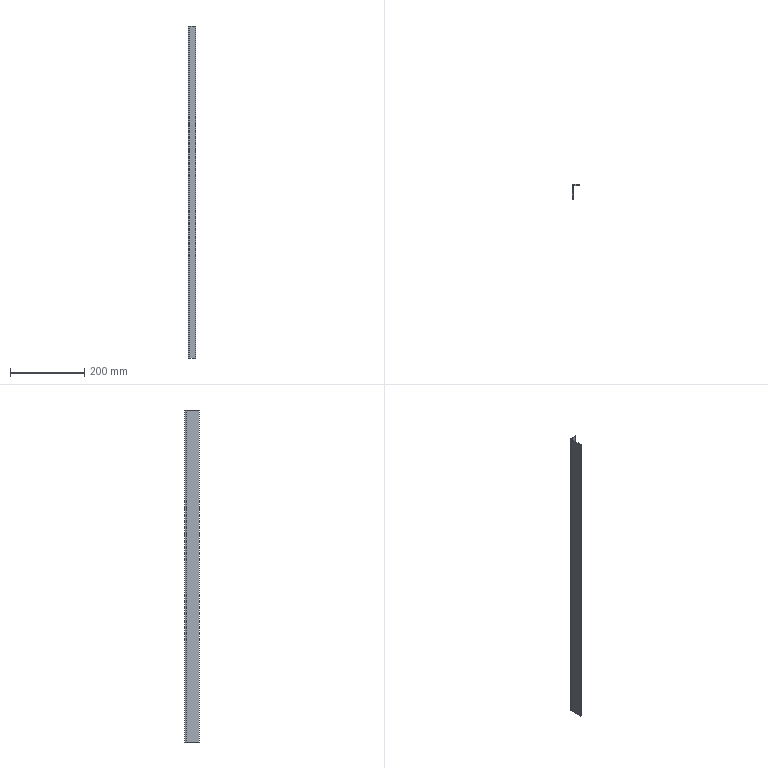Part | SolidWorks | features FlatPattern 1, SMBaseFlange 1, SheetMetal 1 | 1 solid | 14 faces | box 20 x 40 x 895 mm | volume 101515 mm3 | plane 12 | cylinder 2 | commonest cylinder face diameters 4 x1 8 x1
STEP:
#1=CARTESIAN_POINT('',(4.,40.,895.));
#2=VERTEX_POINT('',#1);
#3=CARTESIAN_POINT('',(4.,38.,895.));
#4=VERTEX_POINT('',#3);
#5=CARTESIAN_POINT('',(4.,40.,895.));
#6=DIRECTION('',(0.,-1.,0.));
#7=VECTOR('',#6,1000.);
#8=LINE('',#5,#7);
#9=EDGE_CURVE('',#2,#4,#8,.T.);
#10=ORIENTED_EDGE('',*,*,#9,.F.);
#11=CARTESIAN_POINT('',(0.,36.,895.));
#12=VERTEX_POINT('',#11);
#13=CARTESIAN_POINT('',(4.,36.,895.));
#14=DIRECTION('',(0.,0.,-1.));
#15=DIRECTION('',(1.,0.,0.));
#16=AXIS2_PLACEMENT_3D('',#13,#14,#15);
#17=CIRCLE('',#16,4.);
#18=EDGE_CURVE('',#12,#2,#17,.T.);
#19=ORIENTED_EDGE('',*,*,#18,.F.);
#20=CARTESIAN_POINT('',(2.,36.,895.));
#21=VERTEX_POINT('',#20);
#22=CARTESIAN_POINT('',(2.,36.,895.));
#23=DIRECTION('',(-1.,0.,0.));
#24=VECTOR('',#23,1000.);
#25=LINE('',#22,#24);
#26=EDGE_CURVE('',#21,#12,#25,.T.);
#27=ORIENTED_EDGE('',*,*,#26,.F.);
#28=CARTESIAN_POINT('',(4.,36.,895.));
#29=DIRECTION('',(0.,0.,-1.));
#30=DIRECTION('',(1.,0.,0.));
#31=AXIS2_PLACEMENT_3D('',#28,#29,#30);
#32=CIRCLE('',#31,2.);
#33=EDGE_CURVE('',#21,#4,#32,.T.);
#34=ORIENTED_EDGE('',*,*,#33,.T.);
#35=EDGE_LOOP('',(#10,#19,#27,#34));
#36=FACE_OUTER_BOUND('',#35,.T.);
#37=CARTESIAN_POINT('',(4.,40.,895.));
#38=DIRECTION('',(0.,0.,1.));
#39=DIRECTION('',(1.,0.,0.));
#40=AXIS2_PLACEMENT_3D('',#37,#38,#39);
#41=PLANE('',#40);
#42=ADVANCED_FACE('',(#36),#41,.T.);
#43=CARTESIAN_POINT('',(20.,40.,895.));
#44=VERTEX_POINT('',#43);
#45=CARTESIAN_POINT('',(0.,40.,895.));
#46=DIRECTION('',(1.,0.,0.));
#47=VECTOR('',#46,1000.);
#48=LINE('',#45,#47);
#49=EDGE_CURVE('',#2,#44,#48,.T.);
#50=ORIENTED_EDGE('',*,*,#49,.F.);
#51=ORIENTED_EDGE('',*,*,#9,.T.);
#52=CARTESIAN_POINT('',(20.,38.,895.));
#53=VERTEX_POINT('',#52);
#54=CARTESIAN_POINT('',(0.,38.,895.));
#55=DIRECTION('',(1.,0.,0.));
#56=VECTOR('',#55,1000.);
#57=LINE('',#54,#56);
#58=EDGE_CURVE('',#4,#53,#57,.T.);
#59=ORIENTED_EDGE('',*,*,#58,.T.);
#60=CARTESIAN_POINT('',(20.,40.,895.));
#61=DIRECTION('',(0.,-1.,0.));
#62=VECTOR('',#61,1000.);
#63=LINE('',#60,#62);
#64=EDGE_CURVE('',#44,#53,#63,.T.);
#65=ORIENTED_EDGE('',*,*,#64,.F.);
#66=EDGE_LOOP('',(#50,#51,#59,#65));
#67=FACE_OUTER_BOUND('',#66,.T.);
#68=CARTESIAN_POINT('',(2.,36.,895.));
#69=DIRECTION('',(0.,0.,1.));
#70=DIRECTION('',(1.,0.,0.));
#71=AXIS2_PLACEMENT_3D('',#68,#69,#70);
#72=PLANE('',#71);
#73=ADVANCED_FACE('',(#67),#72,.T.);
#74=CARTESIAN_POINT('',(0.,36.,0.));
#75=VERTEX_POINT('',#74);
#76=CARTESIAN_POINT('',(2.,36.,0.));
#77=VERTEX_POINT('',#76);
#78=CARTESIAN_POINT('',(0.,36.,0.));
#79=DIRECTION('',(1.,0.,0.));
#80=VECTOR('',#79,1000.);
#81=LINE('',#78,#80);
#82=EDGE_CURVE('',#75,#77,#81,.T.);
#83=ORIENTED_EDGE('',*,*,#82,.F.);
#84=CARTESIAN_POINT('',(4.,40.,0.));
#85=VERTEX_POINT('',#84);
#86=CARTESIAN_POINT('',(4.,36.,0.));
#87=DIRECTION('',(0.,0.,-1.));
#88=DIRECTION('',(1.,0.,0.));
#89=AXIS2_PLACEMENT_3D('',#86,#87,#88);
#90=CIRCLE('',#89,4.);
#91=EDGE_CURVE('',#75,#85,#90,.T.);
#92=ORIENTED_EDGE('',*,*,#91,.T.);
#93=CARTESIAN_POINT('',(4.,38.,0.));
#94=VERTEX_POINT('',#93);
#95=CARTESIAN_POINT('',(4.,38.,0.));
#96=DIRECTION('',(0.,1.,0.));
#97=VECTOR('',#96,1000.);
#98=LINE('',#95,#97);
#99=EDGE_CURVE('',#94,#85,#98,.T.);
#100=ORIENTED_EDGE('',*,*,#99,.F.);
#101=CARTESIAN_POINT('',(4.,36.,0.));
#102=DIRECTION('',(0.,0.,-1.));
#103=DIRECTION('',(1.,0.,0.));
#104=AXIS2_PLACEMENT_3D('',#101,#102,#103);
#105=CIRCLE('',#104,2.);
#106=EDGE_CURVE('',#77,#94,#105,.T.);
#107=ORIENTED_EDGE('',*,*,#106,.F.);
#108=EDGE_LOOP('',(#83,#92,#100,#107));
#109=FACE_OUTER_BOUND('',#108,.T.);
#110=CARTESIAN_POINT('',(0.,36.,0.));
#111=DIRECTION('',(0.,0.,-1.));
#112=DIRECTION('',(-1.,0.,0.));
#113=AXIS2_PLACEMENT_3D('',#110,#111,#112);
#114=PLANE('',#113);
#115=ADVANCED_FACE('',(#109),#114,.T.);
#116=CARTESIAN_POINT('',(0.,0.,0.));
#117=VERTEX_POINT('',#116);
#118=CARTESIAN_POINT('',(0.,0.,0.));
#119=DIRECTION('',(0.,1.,0.));
#120=VECTOR('',#119,1000.);
#121=LINE('',#118,#120);
#122=EDGE_CURVE('',#117,#75,#121,.T.);
#123=ORIENTED_EDGE('',*,*,#122,.T.);
#124=ORIENTED_EDGE('',*,*,#82,.T.);
#125=CARTESIAN_POINT('',(2.,0.,0.));
#126=VERTEX_POINT('',#125);
#127=CARTESIAN_POINT('',(2.,0.,0.));
#128=DIRECTION('',(0.,1.,0.));
#129=VECTOR('',#128,1000.);
#130=LINE('',#127,#129);
#131=EDGE_CURVE('',#126,#77,#130,.T.);
#132=ORIENTED_EDGE('',*,*,#131,.F.);
#133=CARTESIAN_POINT('',(2.,0.,0.));
#134=DIRECTION('',(-1.,0.,0.));
#135=VECTOR('',#134,1000.);
#136=LINE('',#133,#135);
#137=EDGE_CURVE('',#126,#117,#136,.T.);
#138=ORIENTED_EDGE('',*,*,#137,.T.);
#139=EDGE_LOOP('',(#123,#124,#132,#138));
#140=FACE_OUTER_BOUND('',#139,.T.);
#141=CARTESIAN_POINT('',(4.,38.,0.));
#142=DIRECTION('',(0.,0.,-1.));
#143=DIRECTION('',(-1.,0.,0.));
#144=AXIS2_PLACEMENT_3D('',#141,#142,#143);
#145=PLANE('',#144);
#146=ADVANCED_FACE('',(#140),#145,.T.);
#147=CARTESIAN_POINT('',(20.,38.,0.));
#148=VERTEX_POINT('',#147);
#149=CARTESIAN_POINT('',(0.,38.,0.));
#150=DIRECTION('',(1.,0.,0.));
#151=VECTOR('',#150,1000.);
#152=LINE('',#149,#151);
#153=EDGE_CURVE('',#94,#148,#152,.T.);
#154=ORIENTED_EDGE('',*,*,#153,.T.);
#155=CARTESIAN_POINT('',(20.,38.,895.));
#156=DIRECTION('',(0.,0.,-1.));
#157=VECTOR('',#156,1000.);
#158=LINE('',#155,#157);
#159=EDGE_CURVE('',#53,#148,#158,.T.);
#160=ORIENTED_EDGE('',*,*,#159,.F.);
#161=ORIENTED_EDGE('',*,*,#58,.F.);
#162=CARTESIAN_POINT('',(4.,38.,895.));
#163=DIRECTION('',(0.,0.,-1.));
#164=VECTOR('',#163,1000.);
#165=LINE('',#162,#164);
#166=EDGE_CURVE('',#4,#94,#165,.T.);
#167=ORIENTED_EDGE('',*,*,#166,.T.);
#168=EDGE_LOOP('',(#154,#160,#161,#167));
#169=FACE_OUTER_BOUND('',#168,.T.);
#170=CARTESIAN_POINT('',(0.,38.,895.));
#171=DIRECTION('',(0.,1.,0.));
#172=DIRECTION('',(0.,0.,1.));
#173=AXIS2_PLACEMENT_3D('',#170,#171,#172);
#174=PLANE('',#173);
#175=ADVANCED_FACE('',(#169),#174,.F.);
#176=CARTESIAN_POINT('',(20.,40.,0.));
#177=VERTEX_POINT('',#176);
#178=CARTESIAN_POINT('',(20.,40.,0.));
#179=DIRECTION('',(0.,-1.,0.));
#180=VECTOR('',#179,1000.);
#181=LINE('',#178,#180);
#182=EDGE_CURVE('',#177,#148,#181,.T.);
#183=ORIENTED_EDGE('',*,*,#182,.F.);
#184=CARTESIAN_POINT('',(20.,40.,895.));
#185=DIRECTION('',(0.,0.,-1.));
#186=VECTOR('',#185,1000.);
#187=LINE('',#184,#186);
#188=EDGE_CURVE('',#44,#177,#187,.T.);
#189=ORIENTED_EDGE('',*,*,#188,.F.);
#190=ORIENTED_EDGE('',*,*,#64,.T.);
#191=ORIENTED_EDGE('',*,*,#159,.T.);
#192=EDGE_LOOP('',(#183,#189,#190,#191));
#193=FACE_OUTER_BOUND('',#192,.T.);
#194=CARTESIAN_POINT('',(20.,40.,895.));
#195=DIRECTION('',(1.,0.,0.));
#196=DIRECTION('',(0.,0.,-1.));
#197=AXIS2_PLACEMENT_3D('',#194,#195,#196);
#198=PLANE('',#197);
#199=ADVANCED_FACE('',(#193),#198,.T.);
#200=CARTESIAN_POINT('',(0.,40.,0.));
#201=DIRECTION('',(1.,0.,0.));
#202=VECTOR('',#201,1000.);
#203=LINE('',#200,#202);
#204=EDGE_CURVE('',#85,#177,#203,.T.);
#205=ORIENTED_EDGE('',*,*,#204,.F.);
#206=CARTESIAN_POINT('',(4.,40.,895.));
#207=DIRECTION('',(0.,0.,-1.));
#208=VECTOR('',#207,1000.);
#209=LINE('',#206,#208);
#210=EDGE_CURVE('',#2,#85,#209,.T.);
#211=ORIENTED_EDGE('',*,*,#210,.F.);
#212=ORIENTED_EDGE('',*,*,#49,.T.);
#213=ORIENTED_EDGE('',*,*,#188,.T.);
#214=EDGE_LOOP('',(#205,#211,#212,#213));
#215=FACE_OUTER_BOUND('',#214,.T.);
#216=CARTESIAN_POINT('',(0.,40.,895.));
#217=DIRECTION('',(0.,1.,0.));
#218=DIRECTION('',(0.,0.,1.));
#219=AXIS2_PLACEMENT_3D('',#216,#217,#218);
#220=PLANE('',#219);
#221=ADVANCED_FACE('',(#215),#220,.T.);
#222=ORIENTED_EDGE('',*,*,#91,.F.);
#223=CARTESIAN_POINT('',(0.,36.,895.));
#224=DIRECTION('',(0.,0.,-1.));
#225=VECTOR('',#224,1000.);
#226=LINE('',#223,#225);
#227=EDGE_CURVE('',#12,#75,#226,.T.);
#228=ORIENTED_EDGE('',*,*,#227,.F.);
#229=ORIENTED_EDGE('',*,*,#18,.T.);
#230=ORIENTED_EDGE('',*,*,#210,.T.);
#231=EDGE_LOOP('',(#222,#228,#229,#230));
#232=FACE_OUTER_BOUND('',#231,.T.);
#233=CARTESIAN_POINT('',(4.,36.,895.));
#234=DIRECTION('',(0.,0.,-1.));
#235=DIRECTION('',(-1.,0.,0.));
#236=AXIS2_PLACEMENT_3D('',#233,#234,#235);
#237=CYLINDRICAL_SURFACE('',#236,4.);
#238=ADVANCED_FACE('',(#232),#237,.T.);
#239=ORIENTED_EDGE('',*,*,#122,.F.);
#240=CARTESIAN_POINT('',(0.,0.,895.));
#241=VERTEX_POINT('',#240);
#242=CARTESIAN_POINT('',(0.,0.,895.));
#243=DIRECTION('',(0.,0.,-1.));
#244=VECTOR('',#243,1000.);
#245=LINE('',#242,#244);
#246=EDGE_CURVE('',#241,#117,#245,.T.);
#247=ORIENTED_EDGE('',*,*,#246,.F.);
#248=CARTESIAN_POINT('',(0.,0.,895.));
#249=DIRECTION('',(0.,1.,0.));
#250=VECTOR('',#249,1000.);
#251=LINE('',#248,#250);
#252=EDGE_CURVE('',#241,#12,#251,.T.);
#253=ORIENTED_EDGE('',*,*,#252,.T.);
#254=ORIENTED_EDGE('',*,*,#227,.T.);
#255=EDGE_LOOP('',(#239,#247,#253,#254));
#256=FACE_OUTER_BOUND('',#255,.T.);
#257=CARTESIAN_POINT('',(0.,0.,895.));
#258=DIRECTION('',(-1.,0.,0.));
#259=DIRECTION('',(0.,0.,1.));
#260=AXIS2_PLACEMENT_3D('',#257,#258,#259);
#261=PLANE('',#260);
#262=ADVANCED_FACE('',(#256),#261,.T.);
#263=ORIENTED_EDGE('',*,*,#137,.F.);
#264=CARTESIAN_POINT('',(2.,0.,895.));
#265=VERTEX_POINT('',#264);
#266=CARTESIAN_POINT('',(2.,0.,895.));
#267=DIRECTION('',(0.,0.,-1.));
#268=VECTOR('',#267,1000.);
#269=LINE('',#266,#268);
#270=EDGE_CURVE('',#265,#126,#269,.T.);
#271=ORIENTED_EDGE('',*,*,#270,.F.);
#272=CARTESIAN_POINT('',(2.,0.,895.));
#273=DIRECTION('',(-1.,0.,0.));
#274=VECTOR('',#273,1000.);
#275=LINE('',#272,#274);
#276=EDGE_CURVE('',#265,#241,#275,.T.);
#277=ORIENTED_EDGE('',*,*,#276,.T.);
#278=ORIENTED_EDGE('',*,*,#246,.T.);
#279=EDGE_LOOP('',(#263,#271,#277,#278));
#280=FACE_OUTER_BOUND('',#279,.T.);
#281=CARTESIAN_POINT('',(2.,0.,895.));
#282=DIRECTION('',(0.,-1.,0.));
#283=DIRECTION('',(0.,0.,-1.));
#284=AXIS2_PLACEMENT_3D('',#281,#282,#283);
#285=PLANE('',#284);
#286=ADVANCED_FACE('',(#280),#285,.T.);
#287=ORIENTED_EDGE('',*,*,#131,.T.);
#288=CARTESIAN_POINT('',(2.,36.,895.));
#289=DIRECTION('',(0.,0.,-1.));
#290=VECTOR('',#289,1000.);
#291=LINE('',#288,#290);
#292=EDGE_CURVE('',#21,#77,#291,.T.);
#293=ORIENTED_EDGE('',*,*,#292,.F.);
#294=CARTESIAN_POINT('',(2.,0.,895.));
#295=DIRECTION('',(0.,1.,0.));
#296=VECTOR('',#295,1000.);
#297=LINE('',#294,#296);
#298=EDGE_CURVE('',#265,#21,#297,.T.);
#299=ORIENTED_EDGE('',*,*,#298,.F.);
#300=ORIENTED_EDGE('',*,*,#270,.T.);
#301=EDGE_LOOP('',(#287,#293,#299,#300));
#302=FACE_OUTER_BOUND('',#301,.T.);
#303=CARTESIAN_POINT('',(2.,0.,895.));
#304=DIRECTION('',(-1.,0.,0.));
#305=DIRECTION('',(0.,0.,1.));
#306=AXIS2_PLACEMENT_3D('',#303,#304,#305);
#307=PLANE('',#306);
#308=ADVANCED_FACE('',(#302),#307,.F.);
#309=ORIENTED_EDGE('',*,*,#106,.T.);
#310=ORIENTED_EDGE('',*,*,#166,.F.);
#311=ORIENTED_EDGE('',*,*,#33,.F.);
#312=ORIENTED_EDGE('',*,*,#292,.T.);
#313=EDGE_LOOP('',(#309,#310,#311,#312));
#314=FACE_OUTER_BOUND('',#313,.T.);
#315=CARTESIAN_POINT('',(4.,36.,895.));
#316=DIRECTION('',(0.,0.,-1.));
#317=DIRECTION('',(-1.,0.,0.));
#318=AXIS2_PLACEMENT_3D('',#315,#316,#317);
#319=CYLINDRICAL_SURFACE('',#318,2.);
#320=ADVANCED_FACE('',(#314),#319,.F.);
#321=ORIENTED_EDGE('',*,*,#298,.T.);
#322=ORIENTED_EDGE('',*,*,#26,.T.);
#323=ORIENTED_EDGE('',*,*,#252,.F.);
#324=ORIENTED_EDGE('',*,*,#276,.F.);
#325=EDGE_LOOP('',(#321,#322,#323,#324));
#326=FACE_OUTER_BOUND('',#325,.T.);
#327=CARTESIAN_POINT('',(4.,36.,895.));
#328=DIRECTION('',(0.,0.,1.));
#329=DIRECTION('',(1.,0.,0.));
#330=AXIS2_PLACEMENT_3D('',#327,#328,#329);
#331=PLANE('',#330);
#332=ADVANCED_FACE('',(#326),#331,.T.);
#333=ORIENTED_EDGE('',*,*,#153,.F.);
#334=ORIENTED_EDGE('',*,*,#99,.T.);
#335=ORIENTED_EDGE('',*,*,#204,.T.);
#336=ORIENTED_EDGE('',*,*,#182,.T.);
#337=EDGE_LOOP('',(#333,#334,#335,#336));
#338=FACE_OUTER_BOUND('',#337,.T.);
#339=CARTESIAN_POINT('',(4.,36.,0.));
#340=DIRECTION('',(0.,0.,1.));
#341=DIRECTION('',(1.,0.,0.));
#342=AXIS2_PLACEMENT_3D('',#339,#340,#341);
#343=PLANE('',#342);
#344=ADVANCED_FACE('',(#338),#343,.F.);
#345=CLOSED_SHELL('',(#42,#73,#115,#146,#175,#199,#221,#238,#262,#286,#308,#320,#332,#344));
#346=MANIFOLD_SOLID_BREP('',#345);
#347=CARTESIAN_POINT('',(0.,0.,0.));
#348=DIRECTION('',(0.,0.,1.));
#349=DIRECTION('',(1.,0.,0.));
#350=AXIS2_PLACEMENT_3D('',#347,#348,#349);
#351=(LENGTH_UNIT()NAMED_UNIT(*)SI_UNIT(.MILLI.,.METRE.));
#352=UNCERTAINTY_MEASURE_WITH_UNIT(LENGTH_MEASURE(0.00001),#351,'','');
#353=(NAMED_UNIT(*)PLANE_ANGLE_UNIT()SI_UNIT($,.RADIAN.));
#354=(NAMED_UNIT(*)SI_UNIT($,.STERADIAN.)SOLID_ANGLE_UNIT());
#355=(GEOMETRIC_REPRESENTATION_CONTEXT(3)GLOBAL_UNCERTAINTY_ASSIGNED_CONTEXT((#352))GLOBAL_UNIT_ASSIGNED_CONTEXT((#351,#353,#354))REPRESENTATION_CONTEXT('',''));
#356=ADVANCED_BREP_SHAPE_REPRESENTATION('',(#346,#350),#355);